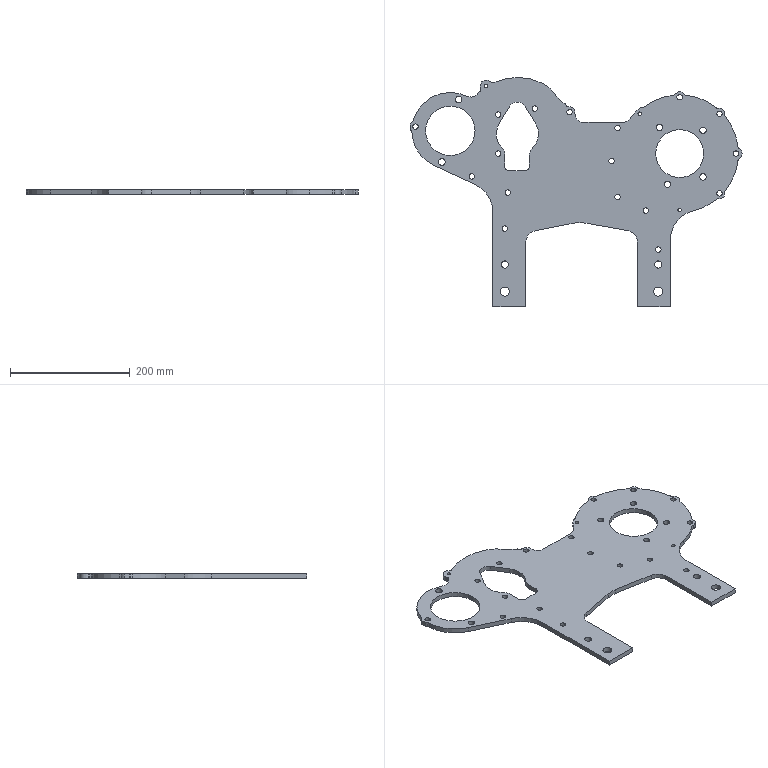Part | SolidWorks | features BaseBody 1 | 1 solid | 138 faces | box 553.5 x 382 x 8 mm | volume 758878 mm3 | cylinder 120 | plane 18 | commonest cylinder face diameters 9 x34 10 x14 10.5 x8 18 x7 6 x6 30 x6